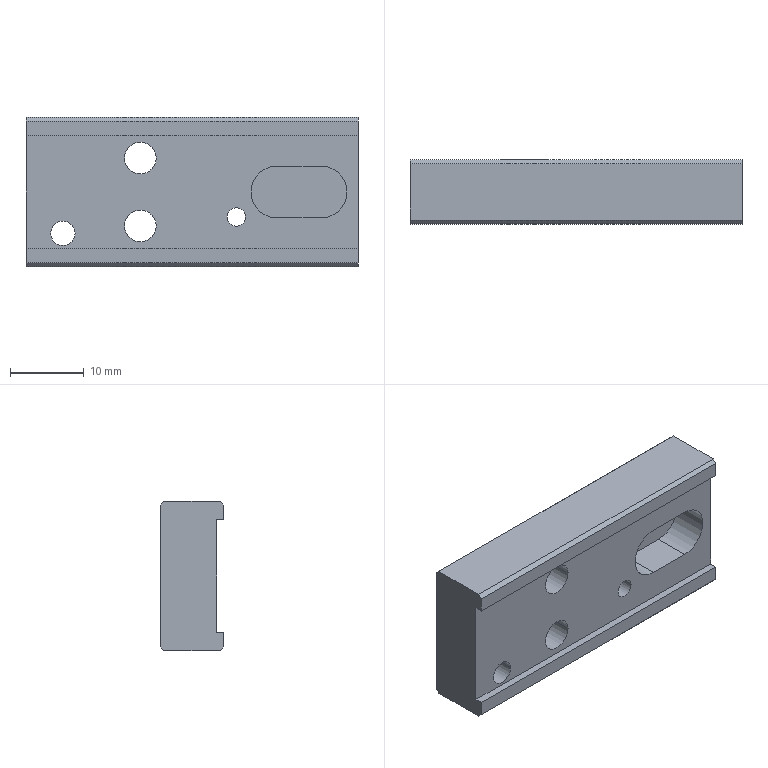Part | NX | 1 solid | 37 faces | box 45 x 8.65 x 20.2 mm | volume 6109 mm3 | plane 19 | cylinder 14 | cone 4 | commonest cylinder face diameters 4.3 x4 8 x4 2.5 x2 3.3 x2 7 x2
STEP:
#1=CARTESIAN_POINT('',(45.,-0.5,0.));
#2=VERTEX_POINT('',#1);
#3=CARTESIAN_POINT('',(0.,-0.5,0.));
#4=VERTEX_POINT('',#3);
#5=CARTESIAN_POINT('',(0.,-0.5,0.));
#6=DIRECTION('',(-1.,0.,0.));
#7=VECTOR('',#6,1000.);
#8=LINE('',#5,#7);
#9=EDGE_CURVE('',#2,#4,#8,.T.);
#10=ORIENTED_EDGE('',*,*,#9,.F.);
#11=CARTESIAN_POINT('',(45.,7.15,0.));
#12=VERTEX_POINT('',#11);
#13=CARTESIAN_POINT('',(45.,-1.,0.));
#14=DIRECTION('',(0.,1.,0.));
#15=VECTOR('',#14,1000.);
#16=LINE('',#13,#15);
#17=EDGE_CURVE('',#2,#12,#16,.T.);
#18=ORIENTED_EDGE('',*,*,#17,.T.);
#19=CARTESIAN_POINT('',(0.,7.15,0.));
#20=VERTEX_POINT('',#19);
#21=CARTESIAN_POINT('',(0.,7.15,0.));
#22=DIRECTION('',(1.,0.,0.));
#23=VECTOR('',#22,1000.);
#24=LINE('',#21,#23);
#25=EDGE_CURVE('',#20,#12,#24,.T.);
#26=ORIENTED_EDGE('',*,*,#25,.F.);
#27=CARTESIAN_POINT('',(0.,7.65,0.));
#28=DIRECTION('',(0.,-1.,0.));
#29=VECTOR('',#28,1000.);
#30=LINE('',#27,#29);
#31=EDGE_CURVE('',#20,#4,#30,.T.);
#32=ORIENTED_EDGE('',*,*,#31,.T.);
#33=EDGE_LOOP('',(#10,#18,#26,#32));
#34=FACE_BOUND('',#33,.T.);
#35=CARTESIAN_POINT('',(0.,0.,0.));
#36=DIRECTION('',(0.,0.,1.));
#37=DIRECTION('',(1.,0.,0.));
#38=AXIS2_PLACEMENT_3D('',#35,#36,#37);
#39=PLANE('',#38);
#40=ADVANCED_FACE('',(#34),#39,.T.);
#41=CARTESIAN_POINT('',(45.,7.15,-20.2));
#42=VERTEX_POINT('',#41);
#43=CARTESIAN_POINT('',(45.,-0.5,-20.2));
#44=VERTEX_POINT('',#43);
#45=CARTESIAN_POINT('',(45.,7.65,-20.2));
#46=DIRECTION('',(0.,-1.,0.));
#47=VECTOR('',#46,1000.);
#48=LINE('',#45,#47);
#49=EDGE_CURVE('',#42,#44,#48,.T.);
#50=ORIENTED_EDGE('',*,*,#49,.F.);
#51=CARTESIAN_POINT('',(45.,7.65,-19.7));
#52=VERTEX_POINT('',#51);
#53=CARTESIAN_POINT('',(45.,27.35,0.));
#54=DIRECTION('',(0.,0.7071,0.7071));
#55=VECTOR('',#54,1000.);
#56=LINE('',#53,#55);
#57=EDGE_CURVE('',#42,#52,#56,.T.);
#58=ORIENTED_EDGE('',*,*,#57,.T.);
#59=CARTESIAN_POINT('',(45.,7.65,-0.5));
#60=VERTEX_POINT('',#59);
#61=CARTESIAN_POINT('',(45.,7.65,0.));
#62=DIRECTION('',(0.,0.,1.));
#63=VECTOR('',#62,1000.);
#64=LINE('',#61,#63);
#65=EDGE_CURVE('',#52,#60,#64,.T.);
#66=ORIENTED_EDGE('',*,*,#65,.T.);
#67=CARTESIAN_POINT('',(45.,7.15,0.));
#68=DIRECTION('',(0.,0.7071,-0.7071));
#69=VECTOR('',#68,1000.);
#70=LINE('',#67,#69);
#71=EDGE_CURVE('',#12,#60,#70,.T.);
#72=ORIENTED_EDGE('',*,*,#71,.F.);
#73=ORIENTED_EDGE('',*,*,#17,.F.);
#74=CARTESIAN_POINT('',(45.,-1.,-0.5));
#75=VERTEX_POINT('',#74);
#76=CARTESIAN_POINT('',(45.,-0.5,0.));
#77=DIRECTION('',(0.,0.7071,0.7071));
#78=VECTOR('',#77,1000.);
#79=LINE('',#76,#78);
#80=EDGE_CURVE('',#75,#2,#79,.T.);
#81=ORIENTED_EDGE('',*,*,#80,.F.);
#82=CARTESIAN_POINT('',(45.,-1.,-2.5));
#83=VERTEX_POINT('',#82);
#84=CARTESIAN_POINT('',(45.,-1.,0.));
#85=DIRECTION('',(0.,0.,-1.));
#86=VECTOR('',#85,1000.);
#87=LINE('',#84,#86);
#88=EDGE_CURVE('',#75,#83,#87,.T.);
#89=ORIENTED_EDGE('',*,*,#88,.T.);
#90=CARTESIAN_POINT('',(45.,0.,-2.5));
#91=VERTEX_POINT('',#90);
#92=CARTESIAN_POINT('',(45.,-1.,-2.5));
#93=DIRECTION('',(0.,1.,0.));
#94=VECTOR('',#93,1000.);
#95=LINE('',#92,#94);
#96=EDGE_CURVE('',#83,#91,#95,.T.);
#97=ORIENTED_EDGE('',*,*,#96,.T.);
#98=CARTESIAN_POINT('',(45.,0.,-17.7));
#99=VERTEX_POINT('',#98);
#100=CARTESIAN_POINT('',(45.,0.,0.));
#101=DIRECTION('',(0.,0.,-1.));
#102=VECTOR('',#101,1000.);
#103=LINE('',#100,#102);
#104=EDGE_CURVE('',#91,#99,#103,.T.);
#105=ORIENTED_EDGE('',*,*,#104,.T.);
#106=CARTESIAN_POINT('',(45.,-1.,-17.7));
#107=VERTEX_POINT('',#106);
#108=CARTESIAN_POINT('',(45.,-1.,-17.7));
#109=DIRECTION('',(0.,1.,0.));
#110=VECTOR('',#109,1000.);
#111=LINE('',#108,#110);
#112=EDGE_CURVE('',#107,#99,#111,.T.);
#113=ORIENTED_EDGE('',*,*,#112,.F.);
#114=CARTESIAN_POINT('',(45.,-1.,-19.7));
#115=VERTEX_POINT('',#114);
#116=CARTESIAN_POINT('',(45.,-1.,-17.7));
#117=DIRECTION('',(0.,0.,-1.));
#118=VECTOR('',#117,1000.);
#119=LINE('',#116,#118);
#120=EDGE_CURVE('',#107,#115,#119,.T.);
#121=ORIENTED_EDGE('',*,*,#120,.T.);
#122=CARTESIAN_POINT('',(45.,-20.7,0.));
#123=DIRECTION('',(0.,-0.7071,0.7071));
#124=VECTOR('',#123,1000.);
#125=LINE('',#122,#124);
#126=EDGE_CURVE('',#44,#115,#125,.T.);
#127=ORIENTED_EDGE('',*,*,#126,.F.);
#128=EDGE_LOOP('',(#50,#58,#66,#72,#73,#81,#89,#97,#105,#113,#121,#127));
#129=FACE_BOUND('',#128,.T.);
#130=CARTESIAN_POINT('',(45.,0.,0.));
#131=DIRECTION('',(1.,0.,0.));
#132=DIRECTION('',(0.,1.,0.));
#133=AXIS2_PLACEMENT_3D('',#130,#131,#132);
#134=PLANE('',#133);
#135=ADVANCED_FACE('',(#129),#134,.T.);
#136=CARTESIAN_POINT('',(0.,-0.5,-20.2));
#137=VERTEX_POINT('',#136);
#138=CARTESIAN_POINT('',(0.,-0.5,-20.2));
#139=DIRECTION('',(-1.,0.,0.));
#140=VECTOR('',#139,1000.);
#141=LINE('',#138,#140);
#142=EDGE_CURVE('',#44,#137,#141,.T.);
#143=ORIENTED_EDGE('',*,*,#142,.T.);
#144=CARTESIAN_POINT('',(0.,7.15,-20.2));
#145=VERTEX_POINT('',#144);
#146=CARTESIAN_POINT('',(0.,-1.,-20.2));
#147=DIRECTION('',(0.,1.,0.));
#148=VECTOR('',#147,1000.);
#149=LINE('',#146,#148);
#150=EDGE_CURVE('',#137,#145,#149,.T.);
#151=ORIENTED_EDGE('',*,*,#150,.T.);
#152=CARTESIAN_POINT('',(0.,7.15,-20.2));
#153=DIRECTION('',(-1.,0.,0.));
#154=VECTOR('',#153,1000.);
#155=LINE('',#152,#154);
#156=EDGE_CURVE('',#42,#145,#155,.T.);
#157=ORIENTED_EDGE('',*,*,#156,.F.);
#158=ORIENTED_EDGE('',*,*,#49,.T.);
#159=EDGE_LOOP('',(#143,#151,#157,#158));
#160=FACE_BOUND('',#159,.T.);
#161=CARTESIAN_POINT('',(0.,0.,-20.2));
#162=DIRECTION('',(0.,0.,1.));
#163=DIRECTION('',(1.,0.,0.));
#164=AXIS2_PLACEMENT_3D('',#161,#162,#163);
#165=PLANE('',#164);
#166=ADVANCED_FACE('',(#160),#165,.F.);
#167=CARTESIAN_POINT('',(0.,0.,-17.7));
#168=VERTEX_POINT('',#167);
#169=CARTESIAN_POINT('',(0.,0.,-2.5));
#170=VERTEX_POINT('',#169);
#171=CARTESIAN_POINT('',(0.,0.,0.));
#172=DIRECTION('',(0.,0.,1.));
#173=VECTOR('',#172,1000.);
#174=LINE('',#171,#173);
#175=EDGE_CURVE('',#168,#170,#174,.T.);
#176=ORIENTED_EDGE('',*,*,#175,.T.);
#177=CARTESIAN_POINT('',(0.,-1.,-2.5));
#178=VERTEX_POINT('',#177);
#179=CARTESIAN_POINT('',(0.,-1.,-2.5));
#180=DIRECTION('',(0.,1.,0.));
#181=VECTOR('',#180,1000.);
#182=LINE('',#179,#181);
#183=EDGE_CURVE('',#178,#170,#182,.T.);
#184=ORIENTED_EDGE('',*,*,#183,.F.);
#185=CARTESIAN_POINT('',(0.,-1.,-0.5));
#186=VERTEX_POINT('',#185);
#187=CARTESIAN_POINT('',(0.,-1.,-2.5));
#188=DIRECTION('',(0.,0.,1.));
#189=VECTOR('',#188,1000.);
#190=LINE('',#187,#189);
#191=EDGE_CURVE('',#178,#186,#190,.T.);
#192=ORIENTED_EDGE('',*,*,#191,.T.);
#193=CARTESIAN_POINT('',(0.,-0.5,0.));
#194=DIRECTION('',(0.,-0.7071,-0.7071));
#195=VECTOR('',#194,1000.);
#196=LINE('',#193,#195);
#197=EDGE_CURVE('',#4,#186,#196,.T.);
#198=ORIENTED_EDGE('',*,*,#197,.F.);
#199=ORIENTED_EDGE('',*,*,#31,.F.);
#200=CARTESIAN_POINT('',(0.,7.65,-0.5));
#201=VERTEX_POINT('',#200);
#202=CARTESIAN_POINT('',(0.,7.15,0.));
#203=DIRECTION('',(0.,-0.7071,0.7071));
#204=VECTOR('',#203,1000.);
#205=LINE('',#202,#204);
#206=EDGE_CURVE('',#201,#20,#205,.T.);
#207=ORIENTED_EDGE('',*,*,#206,.F.);
#208=CARTESIAN_POINT('',(0.,7.65,-19.7));
#209=VERTEX_POINT('',#208);
#210=CARTESIAN_POINT('',(0.,7.65,0.));
#211=DIRECTION('',(0.,0.,-1.));
#212=VECTOR('',#211,1000.);
#213=LINE('',#210,#212);
#214=EDGE_CURVE('',#201,#209,#213,.T.);
#215=ORIENTED_EDGE('',*,*,#214,.T.);
#216=CARTESIAN_POINT('',(0.,27.35,0.));
#217=DIRECTION('',(0.,-0.7071,-0.7071));
#218=VECTOR('',#217,1000.);
#219=LINE('',#216,#218);
#220=EDGE_CURVE('',#209,#145,#219,.T.);
#221=ORIENTED_EDGE('',*,*,#220,.T.);
#222=ORIENTED_EDGE('',*,*,#150,.F.);
#223=CARTESIAN_POINT('',(0.,-1.,-19.7));
#224=VERTEX_POINT('',#223);
#225=CARTESIAN_POINT('',(0.,-20.7,0.));
#226=DIRECTION('',(0.,0.7071,-0.7071));
#227=VECTOR('',#226,1000.);
#228=LINE('',#225,#227);
#229=EDGE_CURVE('',#224,#137,#228,.T.);
#230=ORIENTED_EDGE('',*,*,#229,.F.);
#231=CARTESIAN_POINT('',(0.,-1.,-17.7));
#232=VERTEX_POINT('',#231);
#233=CARTESIAN_POINT('',(0.,-1.,-20.2));
#234=DIRECTION('',(0.,0.,1.));
#235=VECTOR('',#234,1000.);
#236=LINE('',#233,#235);
#237=EDGE_CURVE('',#224,#232,#236,.T.);
#238=ORIENTED_EDGE('',*,*,#237,.T.);
#239=CARTESIAN_POINT('',(0.,-1.,-17.7));
#240=DIRECTION('',(0.,1.,0.));
#241=VECTOR('',#240,1000.);
#242=LINE('',#239,#241);
#243=EDGE_CURVE('',#232,#168,#242,.T.);
#244=ORIENTED_EDGE('',*,*,#243,.T.);
#245=EDGE_LOOP('',(#176,#184,#192,#198,#199,#207,#215,#221,#222,#230,#238,#244));
#246=FACE_BOUND('',#245,.T.);
#247=CARTESIAN_POINT('',(0.,7.65,0.));
#248=DIRECTION('',(-1.,0.,0.));
#249=DIRECTION('',(0.,0.,1.));
#250=AXIS2_PLACEMENT_3D('',#247,#248,#249);
#251=PLANE('',#250);
#252=ADVANCED_FACE('',(#246),#251,.T.);
#253=CARTESIAN_POINT('',(0.,7.65,-0.5));
#254=DIRECTION('',(-1.,0.,0.));
#255=VECTOR('',#254,1000.);
#256=LINE('',#253,#255);
#257=EDGE_CURVE('',#60,#201,#256,.T.);
#258=ORIENTED_EDGE('',*,*,#257,.F.);
#259=ORIENTED_EDGE('',*,*,#65,.F.);
#260=CARTESIAN_POINT('',(0.,7.65,-19.7));
#261=DIRECTION('',(-1.,0.,0.));
#262=VECTOR('',#261,1000.);
#263=LINE('',#260,#262);
#264=EDGE_CURVE('',#52,#209,#263,.T.);
#265=ORIENTED_EDGE('',*,*,#264,.T.);
#266=ORIENTED_EDGE('',*,*,#214,.F.);
#267=EDGE_LOOP('',(#258,#259,#265,#266));
#268=FACE_BOUND('',#267,.T.);
#269=CARTESIAN_POINT('',(19.5,7.65,-14.7));
#270=VERTEX_POINT('',#269);
#271=CARTESIAN_POINT('',(11.5,7.65,-14.7));
#272=VERTEX_POINT('',#271);
#273=CARTESIAN_POINT('',(15.5,7.65,-14.7));
#274=DIRECTION('',(0.,1.,0.));
#275=DIRECTION('',(1.,0.,0.));
#276=AXIS2_PLACEMENT_3D('',#273,#274,#275);
#277=CIRCLE('',#276,4.);
#278=EDGE_CURVE('',#270,#272,#277,.T.);
#279=ORIENTED_EDGE('',*,*,#278,.F.);
#280=CARTESIAN_POINT('',(15.5,7.65,-14.7));
#281=DIRECTION('',(0.,1.,0.));
#282=DIRECTION('',(1.,0.,0.));
#283=AXIS2_PLACEMENT_3D('',#280,#281,#282);
#284=CIRCLE('',#283,4.);
#285=EDGE_CURVE('',#272,#270,#284,.T.);
#286=ORIENTED_EDGE('',*,*,#285,.F.);
#287=EDGE_LOOP('',(#279,#286));
#288=FACE_BOUND('',#287,.T.);
#289=CARTESIAN_POINT('',(7.315,7.65,-15.7));
#290=VERTEX_POINT('',#289);
#291=CARTESIAN_POINT('',(2.685,7.65,-15.7));
#292=VERTEX_POINT('',#291);
#293=CARTESIAN_POINT('',(5.,7.65,-15.7));
#294=DIRECTION('',(0.,1.,0.));
#295=DIRECTION('',(1.,0.,0.));
#296=AXIS2_PLACEMENT_3D('',#293,#294,#295);
#297=CIRCLE('',#296,2.315);
#298=EDGE_CURVE('',#290,#292,#297,.T.);
#299=ORIENTED_EDGE('',*,*,#298,.F.);
#300=CARTESIAN_POINT('',(5.,7.65,-15.7));
#301=DIRECTION('',(0.,1.,0.));
#302=DIRECTION('',(1.,0.,0.));
#303=AXIS2_PLACEMENT_3D('',#300,#301,#302);
#304=CIRCLE('',#303,2.315);
#305=EDGE_CURVE('',#292,#290,#304,.T.);
#306=ORIENTED_EDGE('',*,*,#305,.F.);
#307=EDGE_LOOP('',(#299,#306));
#308=FACE_BOUND('',#307,.T.);
#309=CARTESIAN_POINT('',(19.5,7.65,-5.5));
#310=VERTEX_POINT('',#309);
#311=CARTESIAN_POINT('',(11.5,7.65,-5.5));
#312=VERTEX_POINT('',#311);
#313=CARTESIAN_POINT('',(15.5,7.65,-5.5));
#314=DIRECTION('',(0.,1.,0.));
#315=DIRECTION('',(1.,0.,0.));
#316=AXIS2_PLACEMENT_3D('',#313,#314,#315);
#317=CIRCLE('',#316,4.);
#318=EDGE_CURVE('',#310,#312,#317,.T.);
#319=ORIENTED_EDGE('',*,*,#318,.F.);
#320=CARTESIAN_POINT('',(15.5,7.65,-5.5));
#321=DIRECTION('',(0.,1.,0.));
#322=DIRECTION('',(1.,0.,0.));
#323=AXIS2_PLACEMENT_3D('',#320,#321,#322);
#324=CIRCLE('',#323,4.);
#325=EDGE_CURVE('',#312,#310,#324,.T.);
#326=ORIENTED_EDGE('',*,*,#325,.F.);
#327=EDGE_LOOP('',(#319,#326));
#328=FACE_BOUND('',#327,.T.);
#329=CARTESIAN_POINT('',(30.2,7.65,-13.5));
#330=VERTEX_POINT('',#329);
#331=CARTESIAN_POINT('',(26.8,7.65,-13.5));
#332=VERTEX_POINT('',#331);
#333=CARTESIAN_POINT('',(28.5,7.65,-13.5));
#334=DIRECTION('',(0.,1.,0.));
#335=DIRECTION('',(1.,0.,0.));
#336=AXIS2_PLACEMENT_3D('',#333,#334,#335);
#337=CIRCLE('',#336,1.7);
#338=EDGE_CURVE('',#330,#332,#337,.T.);
#339=ORIENTED_EDGE('',*,*,#338,.F.);
#340=CARTESIAN_POINT('',(28.5,7.65,-13.5));
#341=DIRECTION('',(0.,1.,0.));
#342=DIRECTION('',(1.,0.,0.));
#343=AXIS2_PLACEMENT_3D('',#340,#341,#342);
#344=CIRCLE('',#343,1.7);
#345=EDGE_CURVE('',#332,#330,#344,.T.);
#346=ORIENTED_EDGE('',*,*,#345,.F.);
#347=EDGE_LOOP('',(#339,#346));
#348=FACE_BOUND('',#347,.T.);
#349=CARTESIAN_POINT('',(45.,7.65,0.));
#350=DIRECTION('',(0.,1.,0.));
#351=DIRECTION('',(1.,0.,0.));
#352=AXIS2_PLACEMENT_3D('',#349,#350,#351);
#353=PLANE('',#352);
#354=ADVANCED_FACE('',(#268,#288,#308,#328,#348),#353,.T.);
#355=CARTESIAN_POINT('',(0.,0.,-2.5));
#356=DIRECTION('',(-1.,0.,0.));
#357=VECTOR('',#356,1000.);
#358=LINE('',#355,#357);
#359=EDGE_CURVE('',#91,#170,#358,.T.);
#360=ORIENTED_EDGE('',*,*,#359,.F.);
#361=ORIENTED_EDGE('',*,*,#96,.F.);
#362=CARTESIAN_POINT('',(45.,-1.,-2.5));
#363=DIRECTION('',(-1.,0.,0.));
#364=VECTOR('',#363,1000.);
#365=LINE('',#362,#364);
#366=EDGE_CURVE('',#83,#178,#365,.T.);
#367=ORIENTED_EDGE('',*,*,#366,.T.);
#368=ORIENTED_EDGE('',*,*,#183,.T.);
#369=EDGE_LOOP('',(#360,#361,#367,#368));
#370=FACE_BOUND('',#369,.T.);
#371=CARTESIAN_POINT('',(0.,0.,-2.5));
#372=DIRECTION('',(0.,0.,-1.));
#373=DIRECTION('',(0.,-1.,0.));
#374=AXIS2_PLACEMENT_3D('',#371,#372,#373);
#375=PLANE('',#374);
#376=ADVANCED_FACE('',(#370),#375,.T.);
#377=ORIENTED_EDGE('',*,*,#191,.F.);
#378=ORIENTED_EDGE('',*,*,#366,.F.);
#379=ORIENTED_EDGE('',*,*,#88,.F.);
#380=CARTESIAN_POINT('',(0.,-1.,-0.5));
#381=DIRECTION('',(1.,0.,0.));
#382=VECTOR('',#381,1000.);
#383=LINE('',#380,#382);
#384=EDGE_CURVE('',#186,#75,#383,.T.);
#385=ORIENTED_EDGE('',*,*,#384,.F.);
#386=EDGE_LOOP('',(#377,#378,#379,#385));
#387=FACE_BOUND('',#386,.T.);
#388=CARTESIAN_POINT('',(0.,-1.,0.));
#389=DIRECTION('',(0.,-1.,0.));
#390=DIRECTION('',(0.,0.,-1.));
#391=AXIS2_PLACEMENT_3D('',#388,#389,#390);
#392=PLANE('',#391);
#393=ADVANCED_FACE('',(#387),#392,.T.);
#394=CARTESIAN_POINT('',(0.,0.,-17.7));
#395=DIRECTION('',(1.,0.,0.));
#396=VECTOR('',#395,1000.);
#397=LINE('',#394,#396);
#398=EDGE_CURVE('',#168,#99,#397,.T.);
#399=ORIENTED_EDGE('',*,*,#398,.F.);
#400=ORIENTED_EDGE('',*,*,#243,.F.);
#401=CARTESIAN_POINT('',(0.,-1.,-17.7));
#402=DIRECTION('',(1.,0.,0.));
#403=VECTOR('',#402,1000.);
#404=LINE('',#401,#403);
#405=EDGE_CURVE('',#232,#107,#404,.T.);
#406=ORIENTED_EDGE('',*,*,#405,.T.);
#407=ORIENTED_EDGE('',*,*,#112,.T.);
#408=EDGE_LOOP('',(#399,#400,#406,#407));
#409=FACE_BOUND('',#408,.T.);
#410=CARTESIAN_POINT('',(45.,0.,-17.7));
#411=DIRECTION('',(0.,0.,1.));
#412=DIRECTION('',(1.,0.,0.));
#413=AXIS2_PLACEMENT_3D('',#410,#411,#412);
#414=PLANE('',#413);
#415=ADVANCED_FACE('',(#409),#414,.T.);
#416=CARTESIAN_POINT('',(0.,-1.,-19.7));
#417=DIRECTION('',(-1.,0.,0.));
#418=VECTOR('',#417,1000.);
#419=LINE('',#416,#418);
#420=EDGE_CURVE('',#115,#224,#419,.T.);
#421=ORIENTED_EDGE('',*,*,#420,.F.);
#422=ORIENTED_EDGE('',*,*,#120,.F.);
#423=ORIENTED_EDGE('',*,*,#405,.F.);
#424=ORIENTED_EDGE('',*,*,#237,.F.);
#425=EDGE_LOOP('',(#421,#422,#423,#424));
#426=FACE_BOUND('',#425,.T.);
#427=CARTESIAN_POINT('',(0.,-1.,0.));
#428=DIRECTION('',(0.,-1.,0.));
#429=DIRECTION('',(0.,0.,-1.));
#430=AXIS2_PLACEMENT_3D('',#427,#428,#429);
#431=PLANE('',#430);
#432=ADVANCED_FACE('',(#426),#431,.T.);
#433=CARTESIAN_POINT('',(17.65,0.,-14.7));
#434=VERTEX_POINT('',#433);
#435=CARTESIAN_POINT('',(13.35,0.,-14.7));
#436=VERTEX_POINT('',#435);
#437=CARTESIAN_POINT('',(15.5,0.,-14.7));
#438=DIRECTION('',(0.,1.,0.));
#439=DIRECTION('',(1.,0.,0.));
#440=AXIS2_PLACEMENT_3D('',#437,#438,#439);
#441=CIRCLE('',#440,2.15);
#442=EDGE_CURVE('',#434,#436,#441,.T.);
#443=ORIENTED_EDGE('',*,*,#442,.F.);
#444=CARTESIAN_POINT('',(17.65,3.25,-14.7));
#445=VERTEX_POINT('',#444);
#446=CARTESIAN_POINT('',(17.65,-2.341,-14.7));
#447=DIRECTION('',(0.,1.,0.));
#448=VECTOR('',#447,1000.);
#449=LINE('',#446,#448);
#450=EDGE_CURVE('',#434,#445,#449,.T.);
#451=ORIENTED_EDGE('',*,*,#450,.T.);
#452=CARTESIAN_POINT('',(13.35,3.25,-14.7));
#453=VERTEX_POINT('',#452);
#454=CARTESIAN_POINT('',(15.5,3.25,-14.7));
#455=DIRECTION('',(0.,1.,0.));
#456=DIRECTION('',(-1.,0.,0.));
#457=AXIS2_PLACEMENT_3D('',#454,#455,#456);
#458=CIRCLE('',#457,2.15);
#459=EDGE_CURVE('',#445,#453,#458,.T.);
#460=ORIENTED_EDGE('',*,*,#459,.T.);
#461=CARTESIAN_POINT('',(13.35,-2.341,-14.7));
#462=DIRECTION('',(0.,1.,0.));
#463=VECTOR('',#462,1000.);
#464=LINE('',#461,#463);
#465=EDGE_CURVE('',#436,#453,#464,.T.);
#466=ORIENTED_EDGE('',*,*,#465,.F.);
#467=EDGE_LOOP('',(#443,#451,#460,#466));
#468=FACE_BOUND('',#467,.T.);
#469=CARTESIAN_POINT('',(15.5,-2.341,-14.7));
#470=DIRECTION('',(0.,1.,0.));
#471=DIRECTION('',(1.,0.,0.));
#472=AXIS2_PLACEMENT_3D('',#469,#470,#471);
#473=CYLINDRICAL_SURFACE('',#472,2.15);
#474=ADVANCED_FACE('',(#468),#473,.F.);
#475=ORIENTED_EDGE('',*,*,#318,.T.);
#476=CARTESIAN_POINT('',(11.5,3.15,-5.5));
#477=VERTEX_POINT('',#476);
#478=CARTESIAN_POINT('',(11.5,-2.341,-5.5));
#479=DIRECTION('',(0.,1.,0.));
#480=VECTOR('',#479,1000.);
#481=LINE('',#478,#480);
#482=EDGE_CURVE('',#312,#477,#481,.F.);
#483=ORIENTED_EDGE('',*,*,#482,.T.);
#484=CARTESIAN_POINT('',(19.5,3.15,-5.5));
#485=VERTEX_POINT('',#484);
#486=CARTESIAN_POINT('',(15.5,3.15,-5.5));
#487=DIRECTION('',(0.,-1.,0.));
#488=DIRECTION('',(1.,0.,0.));
#489=AXIS2_PLACEMENT_3D('',#486,#487,#488);
#490=CIRCLE('',#489,4.);
#491=EDGE_CURVE('',#477,#485,#490,.T.);
#492=ORIENTED_EDGE('',*,*,#491,.T.);
#493=CARTESIAN_POINT('',(19.5,-2.341,-5.5));
#494=DIRECTION('',(0.,1.,0.));
#495=VECTOR('',#494,1000.);
#496=LINE('',#493,#495);
#497=EDGE_CURVE('',#310,#485,#496,.F.);
#498=ORIENTED_EDGE('',*,*,#497,.F.);
#499=EDGE_LOOP('',(#475,#483,#492,#498));
#500=FACE_BOUND('',#499,.T.);
#501=CARTESIAN_POINT('',(15.5,-2.341,-5.5));
#502=DIRECTION('',(0.,1.,0.));
#503=DIRECTION('',(1.,0.,0.));
#504=AXIS2_PLACEMENT_3D('',#501,#502,#503);
#505=CYLINDRICAL_SURFACE('',#504,4.);
#506=ADVANCED_FACE('',(#500),#505,.F.);
#507=CARTESIAN_POINT('',(19.5,3.25,-14.7));
#508=VERTEX_POINT('',#507);
#509=CARTESIAN_POINT('',(11.5,3.25,-14.7));
#510=VERTEX_POINT('',#509);
#511=CARTESIAN_POINT('',(15.5,3.25,-14.7));
#512=DIRECTION('',(0.,-1.,0.));
#513=DIRECTION('',(1.,0.,0.));
#514=AXIS2_PLACEMENT_3D('',#511,#512,#513);
#515=CIRCLE('',#514,4.);
#516=EDGE_CURVE('',#508,#510,#515,.T.);
#517=ORIENTED_EDGE('',*,*,#516,.F.);
#518=CARTESIAN_POINT('',(15.5,3.25,-14.7));
#519=DIRECTION('',(0.,-1.,0.));
#520=DIRECTION('',(1.,0.,0.));
#521=AXIS2_PLACEMENT_3D('',#518,#519,#520);
#522=CIRCLE('',#521,4.);
#523=EDGE_CURVE('',#510,#508,#522,.T.);
#524=ORIENTED_EDGE('',*,*,#523,.F.);
#525=EDGE_LOOP('',(#517,#524));
#526=FACE_BOUND('',#525,.T.);
#527=ORIENTED_EDGE('',*,*,#459,.F.);
#528=CARTESIAN_POINT('',(15.5,3.25,-14.7));
#529=DIRECTION('',(0.,1.,0.));
#530=DIRECTION('',(-1.,0.,0.));
#531=AXIS2_PLACEMENT_3D('',#528,#529,#530);
#532=CIRCLE('',#531,2.15);
#533=EDGE_CURVE('',#453,#445,#532,.T.);
#534=ORIENTED_EDGE('',*,*,#533,.F.);
#535=EDGE_LOOP('',(#527,#534));
#536=FACE_BOUND('',#535,.T.);
#537=CARTESIAN_POINT('',(15.5,3.25,-14.7));
#538=DIRECTION('',(0.,1.,0.));
#539=DIRECTION('',(1.,0.,0.));
#540=AXIS2_PLACEMENT_3D('',#537,#538,#539);
#541=PLANE('',#540);
#542=ADVANCED_FACE('',(#526,#536),#541,.T.);
#543=ORIENTED_EDGE('',*,*,#516,.T.);
#544=CARTESIAN_POINT('',(11.5,-2.341,-14.7));
#545=DIRECTION('',(0.,1.,0.));
#546=VECTOR('',#545,1000.);
#547=LINE('',#544,#546);
#548=EDGE_CURVE('',#272,#510,#547,.F.);
#549=ORIENTED_EDGE('',*,*,#548,.F.);
#550=ORIENTED_EDGE('',*,*,#285,.T.);
#551=CARTESIAN_POINT('',(19.5,-2.341,-14.7));
#552=DIRECTION('',(0.,1.,0.));
#553=VECTOR('',#552,1000.);
#554=LINE('',#551,#553);
#555=EDGE_CURVE('',#270,#508,#554,.F.);
#556=ORIENTED_EDGE('',*,*,#555,.T.);
#557=EDGE_LOOP('',(#543,#549,#550,#556));
#558=FACE_BOUND('',#557,.T.);
#559=CARTESIAN_POINT('',(15.5,-2.341,-14.7));
#560=DIRECTION('',(0.,1.,0.));
#561=DIRECTION('',(1.,0.,0.));
#562=AXIS2_PLACEMENT_3D('',#559,#560,#561);
#563=CYLINDRICAL_SURFACE('',#562,4.);
#564=ADVANCED_FACE('',(#558),#563,.F.);
#565=ORIENTED_EDGE('',*,*,#359,.T.);
#566=ORIENTED_EDGE('',*,*,#175,.F.);
#567=ORIENTED_EDGE('',*,*,#398,.T.);
#568=ORIENTED_EDGE('',*,*,#104,.F.);
#569=EDGE_LOOP('',(#565,#566,#567,#568));
#570=FACE_BOUND('',#569,.T.);
#571=ORIENTED_EDGE('',*,*,#442,.T.);
#572=CARTESIAN_POINT('',(15.5,0.,-14.7));
#573=DIRECTION('',(0.,1.,0.));
#574=DIRECTION('',(1.,0.,0.));
#575=AXIS2_PLACEMENT_3D('',#572,#573,#574);
#576=CIRCLE('',#575,2.15);
#577=EDGE_CURVE('',#436,#434,#576,.T.);
#578=ORIENTED_EDGE('',*,*,#577,.T.);
#579=EDGE_LOOP('',(#571,#578));
#580=FACE_BOUND('',#579,.T.);
#581=CARTESIAN_POINT('',(6.65,0.,-15.7));
#582=VERTEX_POINT('',#581);
#583=CARTESIAN_POINT('',(3.35,0.,-15.7));
#584=VERTEX_POINT('',#583);
#585=CARTESIAN_POINT('',(5.,0.,-15.7));
#586=DIRECTION('',(0.,1.,0.));
#587=DIRECTION('',(1.,0.,0.));
#588=AXIS2_PLACEMENT_3D('',#585,#586,#587);
#589=CIRCLE('',#588,1.65);
#590=EDGE_CURVE('',#582,#584,#589,.T.);
#591=ORIENTED_EDGE('',*,*,#590,.T.);
#592=CARTESIAN_POINT('',(5.,0.,-15.7));
#593=DIRECTION('',(0.,1.,0.));
#594=DIRECTION('',(1.,0.,0.));
#595=AXIS2_PLACEMENT_3D('',#592,#593,#594);
#596=CIRCLE('',#595,1.65);
#597=EDGE_CURVE('',#584,#582,#596,.T.);
#598=ORIENTED_EDGE('',*,*,#597,.T.);
#599=EDGE_LOOP('',(#591,#598));
#600=FACE_BOUND('',#599,.T.);
#601=CARTESIAN_POINT('',(29.75,0.,-13.5));
#602=VERTEX_POINT('',#601);
#603=CARTESIAN_POINT('',(27.25,0.,-13.5));
#604=VERTEX_POINT('',#603);
#605=CARTESIAN_POINT('',(28.5,0.,-13.5));
#606=DIRECTION('',(0.,1.,0.));
#607=DIRECTION('',(1.,0.,0.));
#608=AXIS2_PLACEMENT_3D('',#605,#606,#607);
#609=CIRCLE('',#608,1.25);
#610=EDGE_CURVE('',#602,#604,#609,.T.);
#611=ORIENTED_EDGE('',*,*,#610,.T.);
#612=CARTESIAN_POINT('',(28.5,0.,-13.5));
#613=DIRECTION('',(0.,1.,0.));
#614=DIRECTION('',(1.,0.,0.));
#615=AXIS2_PLACEMENT_3D('',#612,#613,#614);
#616=CIRCLE('',#615,1.25);
#617=EDGE_CURVE('',#604,#602,#616,.T.);
#618=ORIENTED_EDGE('',*,*,#617,.T.);
#619=EDGE_LOOP('',(#611,#618));
#620=FACE_BOUND('',#619,.T.);
#621=CARTESIAN_POINT('',(13.35,0.,-5.5));
#622=VERTEX_POINT('',#621);
#623=CARTESIAN_POINT('',(17.65,0.,-5.5));
#624=VERTEX_POINT('',#623);
#625=CARTESIAN_POINT('',(15.5,0.,-5.5));
#626=DIRECTION('',(0.,1.,0.));
#627=DIRECTION('',(1.,0.,0.));
#628=AXIS2_PLACEMENT_3D('',#625,#626,#627);
#629=CIRCLE('',#628,2.15);
#630=EDGE_CURVE('',#622,#624,#629,.T.);
#631=ORIENTED_EDGE('',*,*,#630,.T.);
#632=CARTESIAN_POINT('',(15.5,0.,-5.5));
#633=DIRECTION('',(0.,1.,0.));
#634=DIRECTION('',(1.,0.,0.));
#635=AXIS2_PLACEMENT_3D('',#632,#633,#634);
#636=CIRCLE('',#635,2.15);
#637=EDGE_CURVE('',#624,#622,#636,.T.);
#638=ORIENTED_EDGE('',*,*,#637,.T.);
#639=EDGE_LOOP('',(#631,#638));
#640=FACE_BOUND('',#639,.T.);
#641=CARTESIAN_POINT('',(34.,0.,-6.6));
#642=VERTEX_POINT('',#641);
#643=CARTESIAN_POINT('',(34.,0.,-13.6));
#644=VERTEX_POINT('',#643);
#645=CARTESIAN_POINT('',(34.,0.,-10.1));
#646=DIRECTION('',(0.,-1.,0.));
#647=DIRECTION('',(0.,0.,1.));
#648=AXIS2_PLACEMENT_3D('',#645,#646,#647);
#649=CIRCLE('',#648,3.5);
#650=EDGE_CURVE('',#642,#644,#649,.T.);
#651=ORIENTED_EDGE('',*,*,#650,.F.);
#652=CARTESIAN_POINT('',(40.,0.,-6.6));
#653=VERTEX_POINT('',#652);
#654=CARTESIAN_POINT('',(0.,0.,-6.6));
#655=DIRECTION('',(-1.,0.,0.));
#656=VECTOR('',#655,1000.);
#657=LINE('',#654,#656);
#658=EDGE_CURVE('',#653,#642,#657,.T.);
#659=ORIENTED_EDGE('',*,*,#658,.F.);
#660=CARTESIAN_POINT('',(40.,0.,-13.6));
#661=VERTEX_POINT('',#660);
#662=CARTESIAN_POINT('',(40.,0.,-10.1));
#663=DIRECTION('',(0.,-1.,0.));
#664=DIRECTION('',(0.,0.,1.));
#665=AXIS2_PLACEMENT_3D('',#662,#663,#664);
#666=CIRCLE('',#665,3.5);
#667=EDGE_CURVE('',#661,#653,#666,.T.);
#668=ORIENTED_EDGE('',*,*,#667,.F.);
#669=CARTESIAN_POINT('',(0.,0.,-13.6));
#670=DIRECTION('',(1.,0.,0.));
#671=VECTOR('',#670,1000.);
#672=LINE('',#669,#671);
#673=EDGE_CURVE('',#644,#661,#672,.T.);
#674=ORIENTED_EDGE('',*,*,#673,.F.);
#675=EDGE_LOOP('',(#651,#659,#668,#674));
#676=FACE_BOUND('',#675,.T.);
#677=CARTESIAN_POINT('',(0.,0.,0.));
#678=DIRECTION('',(0.,-1.,0.));
#679=DIRECTION('',(0.,0.,-1.));
#680=AXIS2_PLACEMENT_3D('',#677,#678,#679);
#681=PLANE('',#680);
#682=ADVANCED_FACE('',(#570,#580,#600,#620,#640,#676),#681,.T.);
#683=CARTESIAN_POINT('',(15.5,3.15,-5.5));
#684=DIRECTION('',(0.,-1.,0.));
#685=DIRECTION('',(1.,0.,0.));
#686=AXIS2_PLACEMENT_3D('',#683,#684,#685);
#687=CIRCLE('',#686,4.);
#688=EDGE_CURVE('',#485,#477,#687,.T.);
#689=ORIENTED_EDGE('',*,*,#688,.F.);
#690=ORIENTED_EDGE('',*,*,#491,.F.);
#691=EDGE_LOOP('',(#689,#690));
#692=FACE_BOUND('',#691,.T.);
#693=CARTESIAN_POINT('',(17.65,3.15,-5.5));
#694=VERTEX_POINT('',#693);
#695=CARTESIAN_POINT('',(13.35,3.15,-5.5));
#696=VERTEX_POINT('',#695);
#697=CARTESIAN_POINT('',(15.5,3.15,-5.5));
#698=DIRECTION('',(0.,1.,0.));
#699=DIRECTION('',(1.,0.,0.));
#700=AXIS2_PLACEMENT_3D('',#697,#698,#699);
#701=CIRCLE('',#700,2.15);
#702=EDGE_CURVE('',#694,#696,#701,.T.);
#703=ORIENTED_EDGE('',*,*,#702,.F.);
#704=CARTESIAN_POINT('',(15.5,3.15,-5.5));
#705=DIRECTION('',(0.,1.,0.));
#706=DIRECTION('',(1.,0.,0.));
#707=AXIS2_PLACEMENT_3D('',#704,#705,#706);
#708=CIRCLE('',#707,2.15);
#709=EDGE_CURVE('',#696,#694,#708,.T.);
#710=ORIENTED_EDGE('',*,*,#709,.F.);
#711=EDGE_LOOP('',(#703,#710));
#712=FACE_BOUND('',#711,.T.);
#713=CARTESIAN_POINT('',(15.5,3.15,-5.5));
#714=DIRECTION('',(0.,1.,0.));
#715=DIRECTION('',(1.,0.,0.));
#716=AXIS2_PLACEMENT_3D('',#713,#714,#715);
#717=PLANE('',#716);
#718=ADVANCED_FACE('',(#692,#712),#717,.T.);
#719=ORIENTED_EDGE('',*,*,#702,.T.);
#720=CARTESIAN_POINT('',(13.35,-2.341,-5.5));
#721=DIRECTION('',(0.,1.,0.));
#722=VECTOR('',#721,1000.);
#723=LINE('',#720,#722);
#724=EDGE_CURVE('',#696,#622,#723,.F.);
#725=ORIENTED_EDGE('',*,*,#724,.T.);
#726=ORIENTED_EDGE('',*,*,#637,.F.);
#727=CARTESIAN_POINT('',(17.65,-2.341,-5.5));
#728=DIRECTION('',(0.,1.,0.));
#729=VECTOR('',#728,1000.);
#730=LINE('',#727,#729);
#731=EDGE_CURVE('',#694,#624,#730,.F.);
#732=ORIENTED_EDGE('',*,*,#731,.F.);
#733=EDGE_LOOP('',(#719,#725,#726,#732));
#734=FACE_BOUND('',#733,.T.);
#735=CARTESIAN_POINT('',(15.5,-2.341,-5.5));
#736=DIRECTION('',(0.,1.,0.));
#737=DIRECTION('',(1.,0.,0.));
#738=AXIS2_PLACEMENT_3D('',#735,#736,#737);
#739=CYLINDRICAL_SURFACE('',#738,2.15);
#740=ADVANCED_FACE('',(#734),#739,.F.);
#741=ORIENTED_EDGE('',*,*,#610,.F.);
#742=CARTESIAN_POINT('',(29.75,7.39,-13.5));
#743=VERTEX_POINT('',#742);
#744=CARTESIAN_POINT('',(29.75,7.65,-13.5));
#745=DIRECTION('',(0.,1.,0.));
#746=VECTOR('',#745,1000.);
#747=LINE('',#744,#746);
#748=EDGE_CURVE('',#602,#743,#747,.T.);
#749=ORIENTED_EDGE('',*,*,#748,.T.);
#750=CARTESIAN_POINT('',(27.25,7.39,-13.5));
#751=VERTEX_POINT('',#750);
#752=CARTESIAN_POINT('',(28.5,7.39,-13.5));
#753=DIRECTION('',(0.,1.,0.));
#754=DIRECTION('',(1.,0.,0.));
#755=AXIS2_PLACEMENT_3D('',#752,#753,#754);
#756=CIRCLE('',#755,1.25);
#757=EDGE_CURVE('',#743,#751,#756,.T.);
#758=ORIENTED_EDGE('',*,*,#757,.T.);
#759=CARTESIAN_POINT('',(27.25,7.65,-13.5));
#760=DIRECTION('',(0.,1.,0.));
#761=VECTOR('',#760,1000.);
#762=LINE('',#759,#761);
#763=EDGE_CURVE('',#604,#751,#762,.T.);
#764=ORIENTED_EDGE('',*,*,#763,.F.);
#765=EDGE_LOOP('',(#741,#749,#758,#764));
#766=FACE_BOUND('',#765,.T.);
#767=CARTESIAN_POINT('',(28.5,7.65,-13.5));
#768=DIRECTION('',(0.,1.,0.));
#769=DIRECTION('',(1.,0.,0.));
#770=AXIS2_PLACEMENT_3D('',#767,#768,#769);
#771=CYLINDRICAL_SURFACE('',#770,1.25);
#772=ADVANCED_FACE('',(#766),#771,.F.);
#773=ORIENTED_EDGE('',*,*,#757,.F.);
#774=CARTESIAN_POINT('',(29.75,7.39,-13.5));
#775=DIRECTION('',(0.866,0.5,0.));
#776=VECTOR('',#775,1000.);
#777=LINE('',#774,#776);
#778=EDGE_CURVE('',#743,#330,#777,.T.);
#779=ORIENTED_EDGE('',*,*,#778,.T.);
#780=ORIENTED_EDGE('',*,*,#338,.T.);
#781=CARTESIAN_POINT('',(27.25,7.39,-13.5));
#782=DIRECTION('',(-0.866,0.5,0.));
#783=VECTOR('',#782,1000.);
#784=LINE('',#781,#783);
#785=EDGE_CURVE('',#751,#332,#784,.T.);
#786=ORIENTED_EDGE('',*,*,#785,.F.);
#787=EDGE_LOOP('',(#773,#779,#780,#786));
#788=FACE_BOUND('',#787,.T.);
#789=CARTESIAN_POINT('',(28.5,7.39,-13.5));
#790=DIRECTION('',(0.,1.,0.));
#791=DIRECTION('',(1.,0.,0.));
#792=AXIS2_PLACEMENT_3D('',#789,#790,#791);
#793=CONICAL_SURFACE('',#792,1.25,1.047);
#794=ADVANCED_FACE('',(#788),#793,.F.);
#795=ORIENTED_EDGE('',*,*,#590,.F.);
#796=CARTESIAN_POINT('',(6.65,7.266,-15.7));
#797=VERTEX_POINT('',#796);
#798=CARTESIAN_POINT('',(6.65,7.65,-15.7));
#799=DIRECTION('',(0.,1.,0.));
#800=VECTOR('',#799,1000.);
#801=LINE('',#798,#800);
#802=EDGE_CURVE('',#582,#797,#801,.T.);
#803=ORIENTED_EDGE('',*,*,#802,.T.);
#804=CARTESIAN_POINT('',(3.35,7.266,-15.7));
#805=VERTEX_POINT('',#804);
#806=CARTESIAN_POINT('',(5.,7.266,-15.7));
#807=DIRECTION('',(0.,1.,0.));
#808=DIRECTION('',(1.,0.,0.));
#809=AXIS2_PLACEMENT_3D('',#806,#807,#808);
#810=CIRCLE('',#809,1.65);
#811=EDGE_CURVE('',#797,#805,#810,.T.);
#812=ORIENTED_EDGE('',*,*,#811,.T.);
#813=CARTESIAN_POINT('',(3.35,7.65,-15.7));
#814=DIRECTION('',(0.,1.,0.));
#815=VECTOR('',#814,1000.);
#816=LINE('',#813,#815);
#817=EDGE_CURVE('',#584,#805,#816,.T.);
#818=ORIENTED_EDGE('',*,*,#817,.F.);
#819=EDGE_LOOP('',(#795,#803,#812,#818));
#820=FACE_BOUND('',#819,.T.);
#821=CARTESIAN_POINT('',(5.,7.65,-15.7));
#822=DIRECTION('',(0.,1.,0.));
#823=DIRECTION('',(1.,0.,0.));
#824=AXIS2_PLACEMENT_3D('',#821,#822,#823);
#825=CYLINDRICAL_SURFACE('',#824,1.65);
#826=ADVANCED_FACE('',(#820),#825,.F.);
#827=ORIENTED_EDGE('',*,*,#298,.T.);
#828=CARTESIAN_POINT('',(3.35,7.266,-15.7));
#829=DIRECTION('',(-0.866,0.5,0.));
#830=VECTOR('',#829,1000.);
#831=LINE('',#828,#830);
#832=EDGE_CURVE('',#805,#292,#831,.T.);
#833=ORIENTED_EDGE('',*,*,#832,.F.);
#834=ORIENTED_EDGE('',*,*,#811,.F.);
#835=CARTESIAN_POINT('',(6.65,7.266,-15.7));
#836=DIRECTION('',(0.866,0.5,0.));
#837=VECTOR('',#836,1000.);
#838=LINE('',#835,#837);
#839=EDGE_CURVE('',#797,#290,#838,.T.);
#840=ORIENTED_EDGE('',*,*,#839,.T.);
#841=EDGE_LOOP('',(#827,#833,#834,#840));
#842=FACE_BOUND('',#841,.T.);
#843=CARTESIAN_POINT('',(5.,7.266,-15.7));
#844=DIRECTION('',(0.,1.,0.));
#845=DIRECTION('',(1.,0.,0.));
#846=AXIS2_PLACEMENT_3D('',#843,#844,#845);
#847=CONICAL_SURFACE('',#846,1.65,1.047);
#848=ADVANCED_FACE('',(#842),#847,.F.);
#849=ORIENTED_EDGE('',*,*,#25,.T.);
#850=ORIENTED_EDGE('',*,*,#71,.T.);
#851=ORIENTED_EDGE('',*,*,#257,.T.);
#852=ORIENTED_EDGE('',*,*,#206,.T.);
#853=EDGE_LOOP('',(#849,#850,#851,#852));
#854=FACE_BOUND('',#853,.T.);
#855=CARTESIAN_POINT('',(22.5,7.4,-0.25));
#856=DIRECTION('',(0.,0.7071,0.7071));
#857=DIRECTION('',(1.,0.,0.));
#858=AXIS2_PLACEMENT_3D('',#855,#856,#857);
#859=PLANE('',#858);
#860=ADVANCED_FACE('',(#854),#859,.T.);
#861=ORIENTED_EDGE('',*,*,#9,.T.);
#862=ORIENTED_EDGE('',*,*,#197,.T.);
#863=ORIENTED_EDGE('',*,*,#384,.T.);
#864=ORIENTED_EDGE('',*,*,#80,.T.);
#865=EDGE_LOOP('',(#861,#862,#863,#864));
#866=FACE_BOUND('',#865,.T.);
#867=CARTESIAN_POINT('',(22.5,-0.75,-0.25));
#868=DIRECTION('',(0.,-0.7071,0.7071));
#869=DIRECTION('',(-1.,0.,0.));
#870=AXIS2_PLACEMENT_3D('',#867,#868,#869);
#871=PLANE('',#870);
#872=ADVANCED_FACE('',(#866),#871,.T.);
#873=CARTESIAN_POINT('',(40.,5.,-6.6));
#874=VERTEX_POINT('',#873);
#875=CARTESIAN_POINT('',(40.,0.,-6.6));
#876=DIRECTION('',(0.,-1.,0.));
#877=VECTOR('',#876,1000.);
#878=LINE('',#875,#877);
#879=EDGE_CURVE('',#874,#653,#878,.T.);
#880=ORIENTED_EDGE('',*,*,#879,.F.);
#881=CARTESIAN_POINT('',(40.,5.,-13.6));
#882=VERTEX_POINT('',#881);
#883=CARTESIAN_POINT('',(40.,5.,-10.1));
#884=DIRECTION('',(0.,-1.,0.));
#885=DIRECTION('',(0.,0.,1.));
#886=AXIS2_PLACEMENT_3D('',#883,#884,#885);
#887=CIRCLE('',#886,3.5);
#888=EDGE_CURVE('',#882,#874,#887,.T.);
#889=ORIENTED_EDGE('',*,*,#888,.F.);
#890=CARTESIAN_POINT('',(40.,0.,-13.6));
#891=DIRECTION('',(0.,-1.,0.));
#892=VECTOR('',#891,1000.);
#893=LINE('',#890,#892);
#894=EDGE_CURVE('',#882,#661,#893,.T.);
#895=ORIENTED_EDGE('',*,*,#894,.T.);
#896=ORIENTED_EDGE('',*,*,#667,.T.);
#897=EDGE_LOOP('',(#880,#889,#895,#896));
#898=FACE_BOUND('',#897,.T.);
#899=CARTESIAN_POINT('',(40.,0.,-10.1));
#900=DIRECTION('',(0.,-1.,0.));
#901=DIRECTION('',(0.,0.,1.));
#902=AXIS2_PLACEMENT_3D('',#899,#900,#901);
#903=CYLINDRICAL_SURFACE('',#902,3.5);
#904=ADVANCED_FACE('',(#898),#903,.F.);
#905=CARTESIAN_POINT('',(34.,5.,-6.6));
#906=VERTEX_POINT('',#905);
#907=CARTESIAN_POINT('',(34.,0.,-6.6));
#908=DIRECTION('',(0.,-1.,0.));
#909=VECTOR('',#908,1000.);
#910=LINE('',#907,#909);
#911=EDGE_CURVE('',#906,#642,#910,.T.);
#912=ORIENTED_EDGE('',*,*,#911,.F.);
#913=CARTESIAN_POINT('',(0.,5.,-6.6));
#914=DIRECTION('',(1.,0.,0.));
#915=VECTOR('',#914,1000.);
#916=LINE('',#913,#915);
#917=EDGE_CURVE('',#906,#874,#916,.T.);
#918=ORIENTED_EDGE('',*,*,#917,.T.);
#919=ORIENTED_EDGE('',*,*,#879,.T.);
#920=ORIENTED_EDGE('',*,*,#658,.T.);
#921=EDGE_LOOP('',(#912,#918,#919,#920));
#922=FACE_BOUND('',#921,.T.);
#923=CARTESIAN_POINT('',(40.,0.,-6.6));
#924=DIRECTION('',(0.,0.,1.));
#925=DIRECTION('',(1.,0.,0.));
#926=AXIS2_PLACEMENT_3D('',#923,#924,#925);
#927=PLANE('',#926);
#928=ADVANCED_FACE('',(#922),#927,.F.);
#929=ORIENTED_EDGE('',*,*,#894,.F.);
#930=CARTESIAN_POINT('',(34.,5.,-13.6));
#931=VERTEX_POINT('',#930);
#932=CARTESIAN_POINT('',(0.,5.,-13.6));
#933=DIRECTION('',(-1.,0.,0.));
#934=VECTOR('',#933,1000.);
#935=LINE('',#932,#934);
#936=EDGE_CURVE('',#882,#931,#935,.T.);
#937=ORIENTED_EDGE('',*,*,#936,.T.);
#938=CARTESIAN_POINT('',(34.,0.,-13.6));
#939=DIRECTION('',(0.,-1.,0.));
#940=VECTOR('',#939,1000.);
#941=LINE('',#938,#940);
#942=EDGE_CURVE('',#931,#644,#941,.T.);
#943=ORIENTED_EDGE('',*,*,#942,.T.);
#944=ORIENTED_EDGE('',*,*,#673,.T.);
#945=EDGE_LOOP('',(#929,#937,#943,#944));
#946=FACE_BOUND('',#945,.T.);
#947=CARTESIAN_POINT('',(34.,0.,-13.6));
#948=DIRECTION('',(0.,0.,-1.));
#949=DIRECTION('',(0.,-1.,0.));
#950=AXIS2_PLACEMENT_3D('',#947,#948,#949);
#951=PLANE('',#950);
#952=ADVANCED_FACE('',(#946),#951,.F.);
#953=ORIENTED_EDGE('',*,*,#942,.F.);
#954=CARTESIAN_POINT('',(34.,5.,-10.1));
#955=DIRECTION('',(0.,-1.,0.));
#956=DIRECTION('',(0.,0.,1.));
#957=AXIS2_PLACEMENT_3D('',#954,#955,#956);
#958=CIRCLE('',#957,3.5);
#959=EDGE_CURVE('',#906,#931,#958,.T.);
#960=ORIENTED_EDGE('',*,*,#959,.F.);
#961=ORIENTED_EDGE('',*,*,#911,.T.);
#962=ORIENTED_EDGE('',*,*,#650,.T.);
#963=EDGE_LOOP('',(#953,#960,#961,#962));
#964=FACE_BOUND('',#963,.T.);
#965=CARTESIAN_POINT('',(34.,0.,-10.1));
#966=DIRECTION('',(0.,-1.,0.));
#967=DIRECTION('',(0.,0.,1.));
#968=AXIS2_PLACEMENT_3D('',#965,#966,#967);
#969=CYLINDRICAL_SURFACE('',#968,3.5);
#970=ADVANCED_FACE('',(#964),#969,.F.);
#971=ORIENTED_EDGE('',*,*,#917,.F.);
#972=ORIENTED_EDGE('',*,*,#959,.T.);
#973=ORIENTED_EDGE('',*,*,#936,.F.);
#974=ORIENTED_EDGE('',*,*,#888,.T.);
#975=EDGE_LOOP('',(#971,#972,#973,#974));
#976=FACE_BOUND('',#975,.T.);
#977=CARTESIAN_POINT('',(40.653,5.,-12.821));
#978=DIRECTION('',(0.,-1.,0.));
#979=DIRECTION('',(0.,0.,-1.));
#980=AXIS2_PLACEMENT_3D('',#977,#978,#979);
#981=PLANE('',#980);
#982=ADVANCED_FACE('',(#976),#981,.T.);
#983=ORIENTED_EDGE('',*,*,#156,.T.);
#984=ORIENTED_EDGE('',*,*,#220,.F.);
#985=ORIENTED_EDGE('',*,*,#264,.F.);
#986=ORIENTED_EDGE('',*,*,#57,.F.);
#987=EDGE_LOOP('',(#983,#984,#985,#986));
#988=FACE_BOUND('',#987,.T.);
#989=CARTESIAN_POINT('',(22.5,7.4,-19.95));
#990=DIRECTION('',(0.,-0.7071,0.7071));
#991=DIRECTION('',(-1.,0.,0.));
#992=AXIS2_PLACEMENT_3D('',#989,#990,#991);
#993=PLANE('',#992);
#994=ADVANCED_FACE('',(#988),#993,.F.);
#995=ORIENTED_EDGE('',*,*,#142,.F.);
#996=ORIENTED_EDGE('',*,*,#126,.T.);
#997=ORIENTED_EDGE('',*,*,#420,.T.);
#998=ORIENTED_EDGE('',*,*,#229,.T.);
#999=EDGE_LOOP('',(#995,#996,#997,#998));
#1000=FACE_BOUND('',#999,.T.);
#1001=CARTESIAN_POINT('',(22.5,-0.75,-19.95));
#1002=DIRECTION('',(0.,-0.7071,-0.7071));
#1003=DIRECTION('',(0.,-0.7071,0.7071));
#1004=AXIS2_PLACEMENT_3D('',#1001,#1002,#1003);
#1005=PLANE('',#1004);
#1006=ADVANCED_FACE('',(#1000),#1005,.T.);
#1007=ORIENTED_EDGE('',*,*,#630,.F.);
#1008=ORIENTED_EDGE('',*,*,#724,.F.);
#1009=ORIENTED_EDGE('',*,*,#709,.T.);
#1010=ORIENTED_EDGE('',*,*,#731,.T.);
#1011=EDGE_LOOP('',(#1007,#1008,#1009,#1010));
#1012=FACE_BOUND('',#1011,.T.);
#1013=CARTESIAN_POINT('',(15.5,-2.341,-5.5));
#1014=DIRECTION('',(0.,1.,0.));
#1015=DIRECTION('',(1.,0.,0.));
#1016=AXIS2_PLACEMENT_3D('',#1013,#1014,#1015);
#1017=CYLINDRICAL_SURFACE('',#1016,2.15);
#1018=ADVANCED_FACE('',(#1012),#1017,.F.);
#1019=ORIENTED_EDGE('',*,*,#278,.T.);
#1020=ORIENTED_EDGE('',*,*,#548,.T.);
#1021=ORIENTED_EDGE('',*,*,#523,.T.);
#1022=ORIENTED_EDGE('',*,*,#555,.F.);
#1023=EDGE_LOOP('',(#1019,#1020,#1021,#1022));
#1024=FACE_BOUND('',#1023,.T.);
#1025=CARTESIAN_POINT('',(15.5,-2.341,-14.7));
#1026=DIRECTION('',(0.,1.,0.));
#1027=DIRECTION('',(1.,0.,0.));
#1028=AXIS2_PLACEMENT_3D('',#1025,#1026,#1027);
#1029=CYLINDRICAL_SURFACE('',#1028,4.);
#1030=ADVANCED_FACE('',(#1024),#1029,.F.);
#1031=ORIENTED_EDGE('',*,*,#688,.T.);
#1032=ORIENTED_EDGE('',*,*,#482,.F.);
#1033=ORIENTED_EDGE('',*,*,#325,.T.);
#1034=ORIENTED_EDGE('',*,*,#497,.T.);
#1035=EDGE_LOOP('',(#1031,#1032,#1033,#1034));
#1036=FACE_BOUND('',#1035,.T.);
#1037=CARTESIAN_POINT('',(15.5,-2.341,-5.5));
#1038=DIRECTION('',(0.,1.,0.));
#1039=DIRECTION('',(1.,0.,0.));
#1040=AXIS2_PLACEMENT_3D('',#1037,#1038,#1039);
#1041=CYLINDRICAL_SURFACE('',#1040,4.);
#1042=ADVANCED_FACE('',(#1036),#1041,.F.);
#1043=ORIENTED_EDGE('',*,*,#450,.F.);
#1044=ORIENTED_EDGE('',*,*,#577,.F.);
#1045=ORIENTED_EDGE('',*,*,#465,.T.);
#1046=ORIENTED_EDGE('',*,*,#533,.T.);
#1047=EDGE_LOOP('',(#1043,#1044,#1045,#1046));
#1048=FACE_BOUND('',#1047,.T.);
#1049=CARTESIAN_POINT('',(15.5,-2.341,-14.7));
#1050=DIRECTION('',(0.,1.,0.));
#1051=DIRECTION('',(1.,0.,0.));
#1052=AXIS2_PLACEMENT_3D('',#1049,#1050,#1051);
#1053=CYLINDRICAL_SURFACE('',#1052,2.15);
#1054=ADVANCED_FACE('',(#1048),#1053,.F.);
#1055=ORIENTED_EDGE('',*,*,#802,.F.);
#1056=ORIENTED_EDGE('',*,*,#597,.F.);
#1057=ORIENTED_EDGE('',*,*,#817,.T.);
#1058=CARTESIAN_POINT('',(5.,7.266,-15.7));
#1059=DIRECTION('',(0.,1.,0.));
#1060=DIRECTION('',(1.,0.,0.));
#1061=AXIS2_PLACEMENT_3D('',#1058,#1059,#1060);
#1062=CIRCLE('',#1061,1.65);
#1063=EDGE_CURVE('',#805,#797,#1062,.T.);
#1064=ORIENTED_EDGE('',*,*,#1063,.T.);
#1065=EDGE_LOOP('',(#1055,#1056,#1057,#1064));
#1066=FACE_BOUND('',#1065,.T.);
#1067=CARTESIAN_POINT('',(5.,7.65,-15.7));
#1068=DIRECTION('',(0.,1.,0.));
#1069=DIRECTION('',(1.,0.,0.));
#1070=AXIS2_PLACEMENT_3D('',#1067,#1068,#1069);
#1071=CYLINDRICAL_SURFACE('',#1070,1.65);
#1072=ADVANCED_FACE('',(#1066),#1071,.F.);
#1073=ORIENTED_EDGE('',*,*,#839,.F.);
#1074=ORIENTED_EDGE('',*,*,#1063,.F.);
#1075=ORIENTED_EDGE('',*,*,#832,.T.);
#1076=ORIENTED_EDGE('',*,*,#305,.T.);
#1077=EDGE_LOOP('',(#1073,#1074,#1075,#1076));
#1078=FACE_BOUND('',#1077,.T.);
#1079=CARTESIAN_POINT('',(5.,7.266,-15.7));
#1080=DIRECTION('',(0.,1.,0.));
#1081=DIRECTION('',(1.,0.,0.));
#1082=AXIS2_PLACEMENT_3D('',#1079,#1080,#1081);
#1083=CONICAL_SURFACE('',#1082,1.65,1.047);
#1084=ADVANCED_FACE('',(#1078),#1083,.F.);
#1085=ORIENTED_EDGE('',*,*,#748,.F.);
#1086=ORIENTED_EDGE('',*,*,#617,.F.);
#1087=ORIENTED_EDGE('',*,*,#763,.T.);
#1088=CARTESIAN_POINT('',(28.5,7.39,-13.5));
#1089=DIRECTION('',(0.,1.,0.));
#1090=DIRECTION('',(1.,0.,0.));
#1091=AXIS2_PLACEMENT_3D('',#1088,#1089,#1090);
#1092=CIRCLE('',#1091,1.25);
#1093=EDGE_CURVE('',#751,#743,#1092,.T.);
#1094=ORIENTED_EDGE('',*,*,#1093,.T.);
#1095=EDGE_LOOP('',(#1085,#1086,#1087,#1094));
#1096=FACE_BOUND('',#1095,.T.);
#1097=CARTESIAN_POINT('',(28.5,7.65,-13.5));
#1098=DIRECTION('',(0.,1.,0.));
#1099=DIRECTION('',(1.,0.,0.));
#1100=AXIS2_PLACEMENT_3D('',#1097,#1098,#1099);
#1101=CYLINDRICAL_SURFACE('',#1100,1.25);
#1102=ADVANCED_FACE('',(#1096),#1101,.F.);
#1103=ORIENTED_EDGE('',*,*,#778,.F.);
#1104=ORIENTED_EDGE('',*,*,#1093,.F.);
#1105=ORIENTED_EDGE('',*,*,#785,.T.);
#1106=ORIENTED_EDGE('',*,*,#345,.T.);
#1107=EDGE_LOOP('',(#1103,#1104,#1105,#1106));
#1108=FACE_BOUND('',#1107,.T.);
#1109=CARTESIAN_POINT('',(28.5,7.39,-13.5));
#1110=DIRECTION('',(0.,1.,0.));
#1111=DIRECTION('',(1.,0.,0.));
#1112=AXIS2_PLACEMENT_3D('',#1109,#1110,#1111);
#1113=CONICAL_SURFACE('',#1112,1.25,1.047);
#1114=ADVANCED_FACE('',(#1108),#1113,.F.);
#1115=CLOSED_SHELL('',(#40,#135,#166,#252,#354,#376,#393,#415,#432,#474,#506,#542,#564,#682,#718,#740,#772,#794,#826,#848,#860,#872,#904,#928,#952,#970,#982,#994,#1006,#1018,#1030,#1042,#1054,#1072,#1084,#1102,#1114));
#1116=MANIFOLD_SOLID_BREP('',#1115);
#1117=(LENGTH_UNIT()NAMED_UNIT(*)SI_UNIT(.MILLI.,.METRE.));
#1118=UNCERTAINTY_MEASURE_WITH_UNIT(LENGTH_MEASURE(0.00001),#1117,'','');
#1119=(NAMED_UNIT(*)PLANE_ANGLE_UNIT()SI_UNIT($,.RADIAN.));
#1120=(NAMED_UNIT(*)SI_UNIT($,.STERADIAN.)SOLID_ANGLE_UNIT());
#1121=(GEOMETRIC_REPRESENTATION_CONTEXT(3)GLOBAL_UNCERTAINTY_ASSIGNED_CONTEXT((#1118))GLOBAL_UNIT_ASSIGNED_CONTEXT((#1117,#1119,#1120))REPRESENTATION_CONTEXT('',''));
#1122=ADVANCED_BREP_SHAPE_REPRESENTATION('',(#1116),#1121);